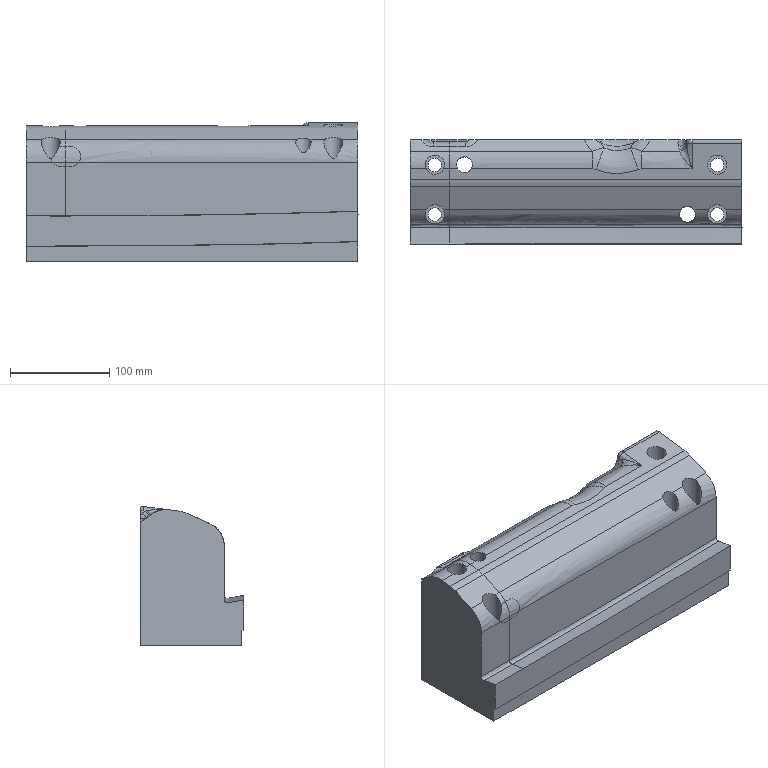Part | NX | features solid 2 | 1 solid | 74 faces | box 335 x 104.851 x 140.327 mm | volume 3788230 mm3 | spline 56 | cylinder 10 | plane 8 | commonest cylinder face diameters 13.5 x4 19.5 x4 16 x2